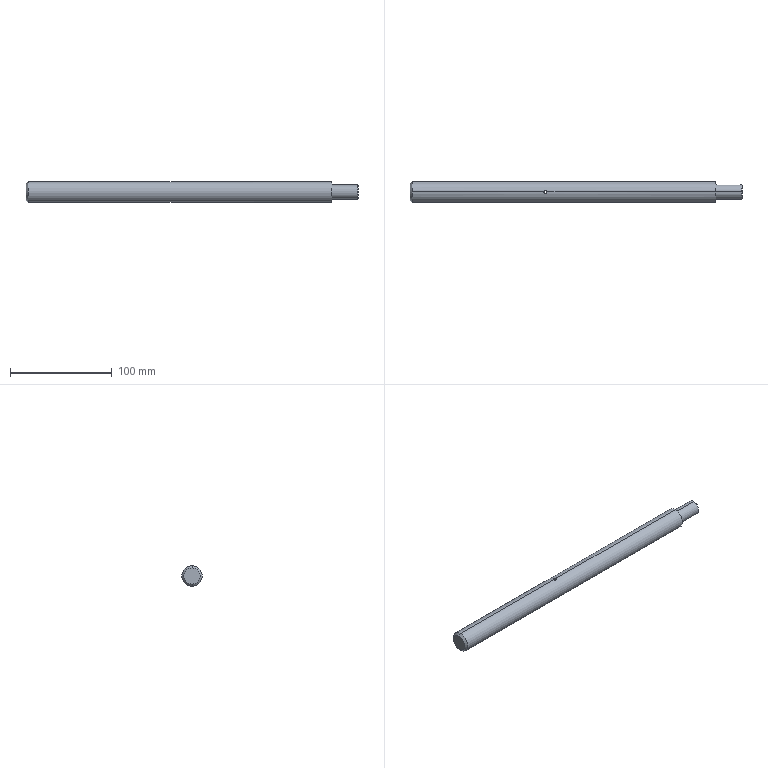Part | STEP file | height adjusting screw rod 2A_SUS304 | 1 solid | 18 faces | box 326 x 20 x 20 mm | volume 97813 mm3 | cylinder 8 | plane 6 | cone 4 | commonest cylinder face diameters 3 x2 4 x2 14 x2 20 x2